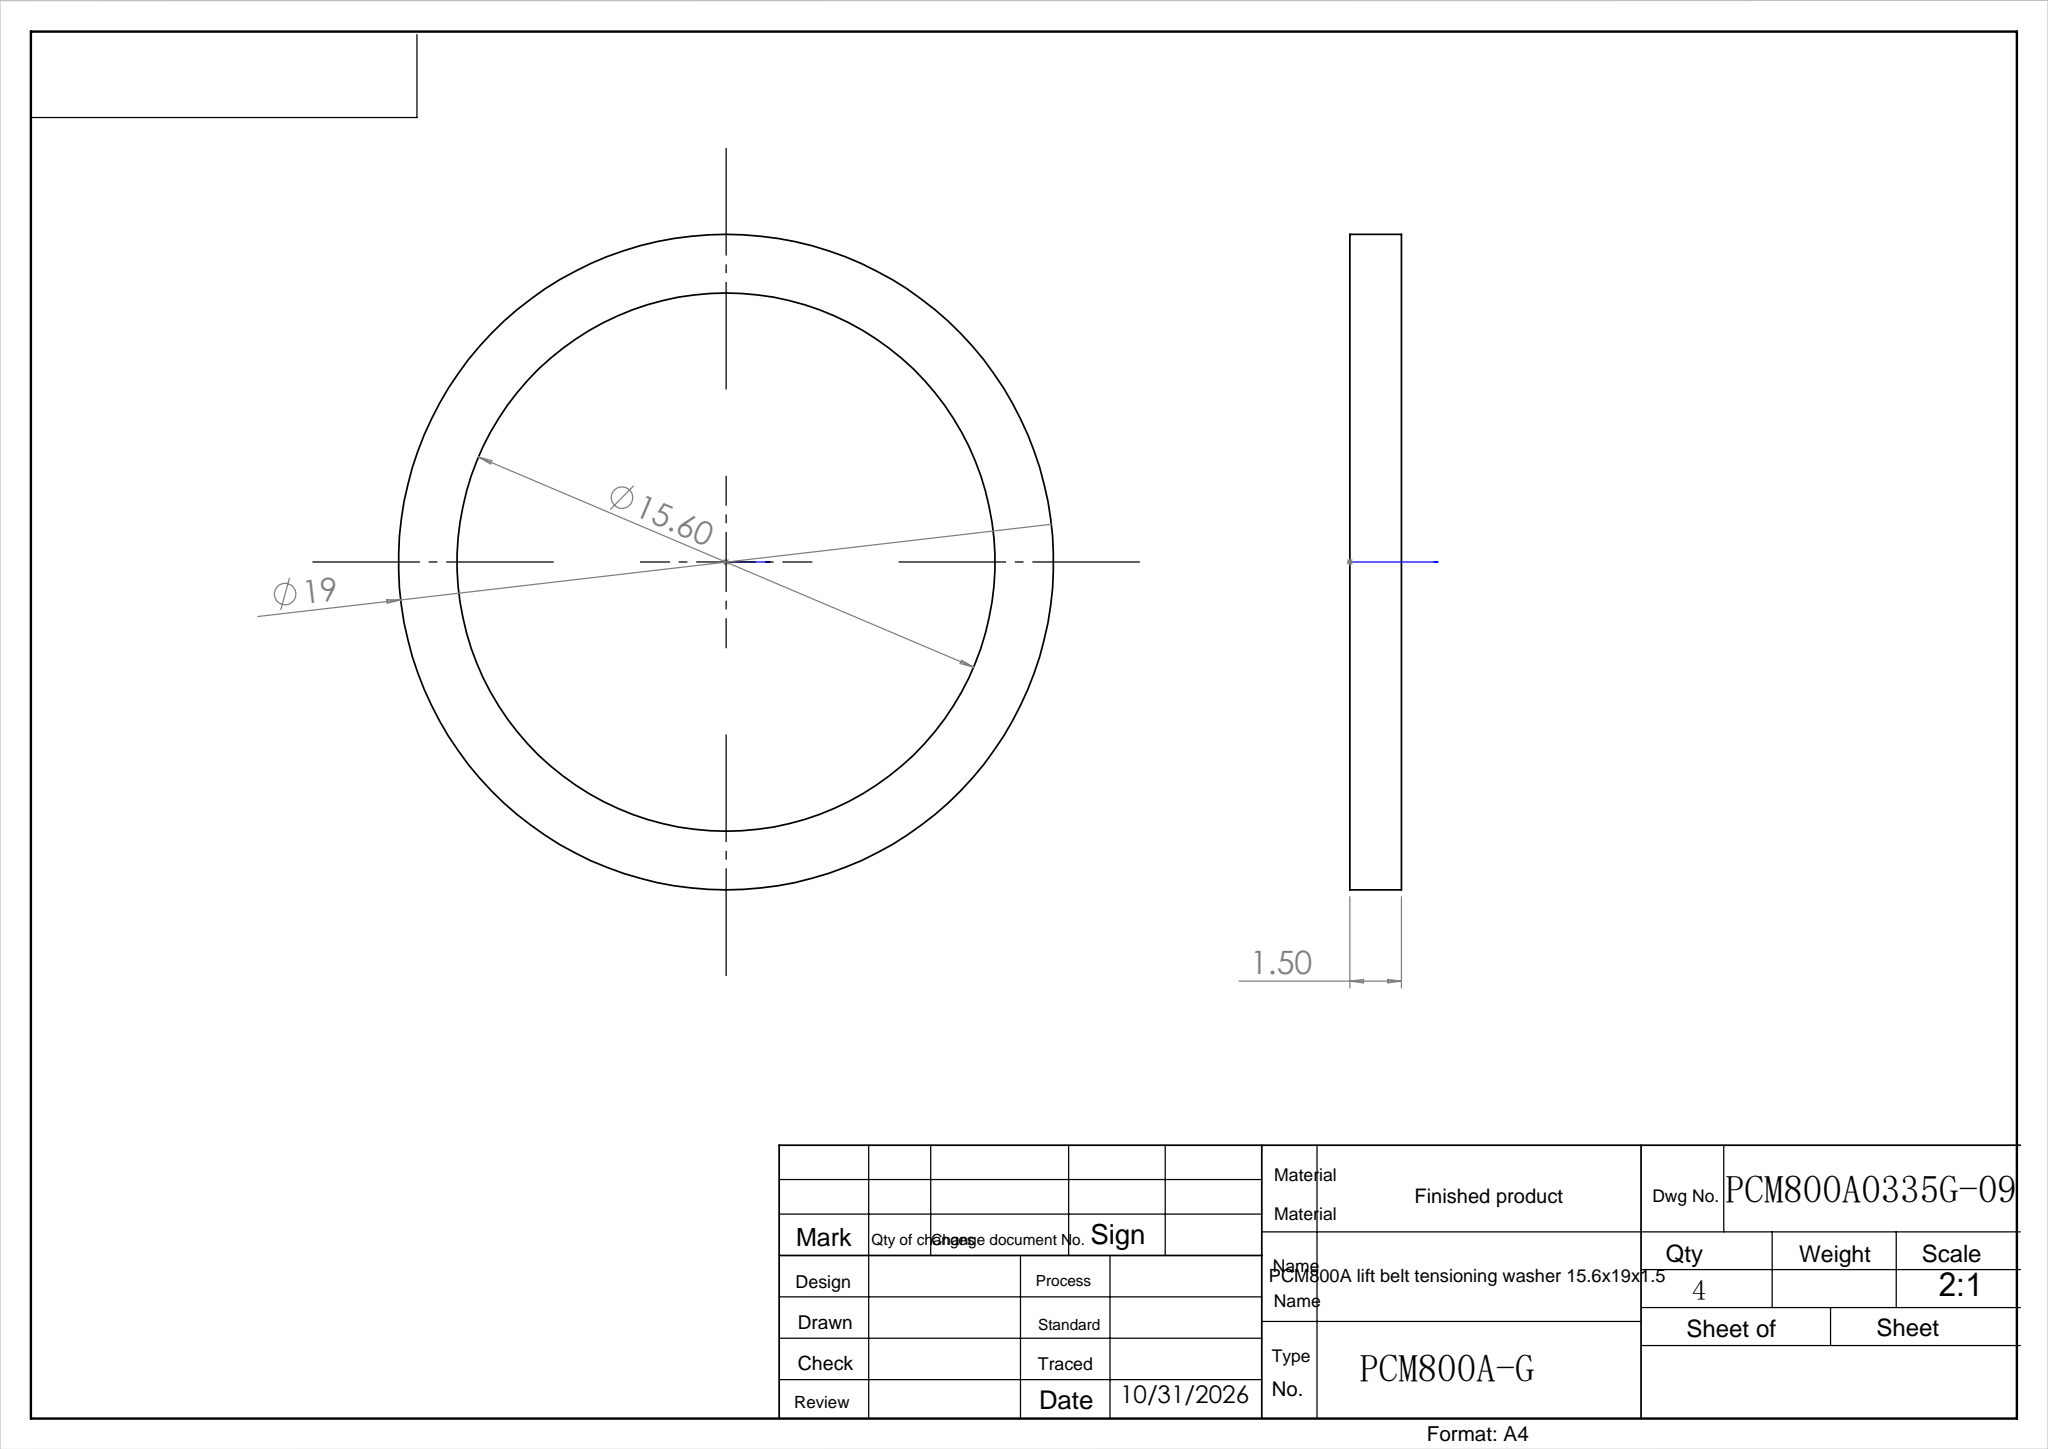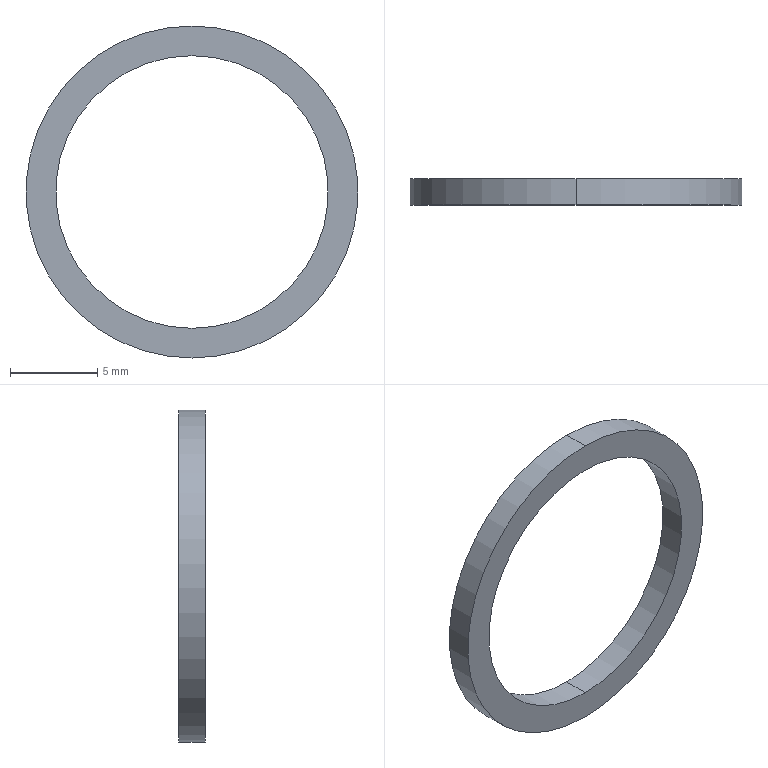Part | SolidWorks | features Extrusion 1 | 1 solid | 6 faces | box 19 x 1.5 x 19 mm | volume 138.591 mm3 | cylinder 4 | plane 2 | commonest cylinder face diameters 15.6 x2 19 x2
STEP:
#1=CARTESIAN_POINT('',(0.,1.5,-7.8));
#2=VERTEX_POINT('',#1);
#3=CARTESIAN_POINT('',(0.,1.5,7.8));
#4=VERTEX_POINT('',#3);
#5=CARTESIAN_POINT('',(0.,1.5,0.));
#6=DIRECTION('',(0.,1.,0.));
#7=DIRECTION('',(0.,0.,1.));
#8=AXIS2_PLACEMENT_3D('',#5,#6,#7);
#9=CIRCLE('',#8,7.8);
#10=EDGE_CURVE('',#2,#4,#9,.T.);
#11=ORIENTED_EDGE('',*,*,#10,.T.);
#12=CARTESIAN_POINT('',(0.,0.,7.8));
#13=VERTEX_POINT('',#12);
#14=CARTESIAN_POINT('',(0.,1.5,7.8));
#15=DIRECTION('',(0.,-1.,0.));
#16=VECTOR('',#15,1000.);
#17=LINE('',#14,#16);
#18=EDGE_CURVE('',#4,#13,#17,.T.);
#19=ORIENTED_EDGE('',*,*,#18,.T.);
#20=CARTESIAN_POINT('',(0.,0.,-7.8));
#21=VERTEX_POINT('',#20);
#22=CARTESIAN_POINT('',(0.,0.,0.));
#23=DIRECTION('',(0.,1.,0.));
#24=DIRECTION('',(0.,0.,1.));
#25=AXIS2_PLACEMENT_3D('',#22,#23,#24);
#26=CIRCLE('',#25,7.8);
#27=EDGE_CURVE('',#21,#13,#26,.T.);
#28=ORIENTED_EDGE('',*,*,#27,.F.);
#29=CARTESIAN_POINT('',(0.,1.5,-7.8));
#30=DIRECTION('',(0.,-1.,0.));
#31=VECTOR('',#30,1000.);
#32=LINE('',#29,#31);
#33=EDGE_CURVE('',#2,#21,#32,.T.);
#34=ORIENTED_EDGE('',*,*,#33,.F.);
#35=EDGE_LOOP('',(#11,#19,#28,#34));
#36=FACE_OUTER_BOUND('',#35,.T.);
#37=CARTESIAN_POINT('',(0.,1.5,0.));
#38=DIRECTION('',(0.,-1.,0.));
#39=DIRECTION('',(0.,0.,-1.));
#40=AXIS2_PLACEMENT_3D('',#37,#38,#39);
#41=CYLINDRICAL_SURFACE('',#40,7.8);
#42=ADVANCED_FACE('',(#36),#41,.F.);
#43=CARTESIAN_POINT('',(0.,1.5,9.5));
#44=VERTEX_POINT('',#43);
#45=CARTESIAN_POINT('',(0.,1.5,-9.5));
#46=VERTEX_POINT('',#45);
#47=CARTESIAN_POINT('',(0.,1.5,0.));
#48=DIRECTION('',(0.,1.,0.));
#49=DIRECTION('',(0.,0.,1.));
#50=AXIS2_PLACEMENT_3D('',#47,#48,#49);
#51=CIRCLE('',#50,9.5);
#52=EDGE_CURVE('',#44,#46,#51,.T.);
#53=ORIENTED_EDGE('',*,*,#52,.F.);
#54=CARTESIAN_POINT('',(0.,0.,9.5));
#55=VERTEX_POINT('',#54);
#56=CARTESIAN_POINT('',(0.,1.5,9.5));
#57=DIRECTION('',(0.,-1.,0.));
#58=VECTOR('',#57,1000.);
#59=LINE('',#56,#58);
#60=EDGE_CURVE('',#44,#55,#59,.T.);
#61=ORIENTED_EDGE('',*,*,#60,.T.);
#62=CARTESIAN_POINT('',(0.,0.,-9.5));
#63=VERTEX_POINT('',#62);
#64=CARTESIAN_POINT('',(0.,0.,0.));
#65=DIRECTION('',(0.,1.,0.));
#66=DIRECTION('',(0.,0.,1.));
#67=AXIS2_PLACEMENT_3D('',#64,#65,#66);
#68=CIRCLE('',#67,9.5);
#69=EDGE_CURVE('',#55,#63,#68,.T.);
#70=ORIENTED_EDGE('',*,*,#69,.T.);
#71=CARTESIAN_POINT('',(0.,1.5,-9.5));
#72=DIRECTION('',(0.,-1.,0.));
#73=VECTOR('',#72,1000.);
#74=LINE('',#71,#73);
#75=EDGE_CURVE('',#46,#63,#74,.T.);
#76=ORIENTED_EDGE('',*,*,#75,.F.);
#77=EDGE_LOOP('',(#53,#61,#70,#76));
#78=FACE_OUTER_BOUND('',#77,.T.);
#79=CARTESIAN_POINT('',(0.,1.5,0.));
#80=DIRECTION('',(0.,-1.,0.));
#81=DIRECTION('',(0.,0.,-1.));
#82=AXIS2_PLACEMENT_3D('',#79,#80,#81);
#83=CYLINDRICAL_SURFACE('',#82,9.5);
#84=ADVANCED_FACE('',(#78),#83,.T.);
#85=CARTESIAN_POINT('',(0.,1.5,0.));
#86=DIRECTION('',(0.,1.,0.));
#87=DIRECTION('',(0.,0.,1.));
#88=AXIS2_PLACEMENT_3D('',#85,#86,#87);
#89=CIRCLE('',#88,9.5);
#90=EDGE_CURVE('',#46,#44,#89,.T.);
#91=ORIENTED_EDGE('',*,*,#90,.T.);
#92=ORIENTED_EDGE('',*,*,#52,.T.);
#93=EDGE_LOOP('',(#91,#92));
#94=FACE_OUTER_BOUND('',#93,.T.);
#95=ORIENTED_EDGE('',*,*,#10,.F.);
#96=CARTESIAN_POINT('',(0.,1.5,0.));
#97=DIRECTION('',(0.,1.,0.));
#98=DIRECTION('',(0.,0.,1.));
#99=AXIS2_PLACEMENT_3D('',#96,#97,#98);
#100=CIRCLE('',#99,7.8);
#101=EDGE_CURVE('',#4,#2,#100,.T.);
#102=ORIENTED_EDGE('',*,*,#101,.F.);
#103=EDGE_LOOP('',(#95,#102));
#104=FACE_BOUND('',#103,.T.);
#105=CARTESIAN_POINT('',(0.,1.5,0.));
#106=DIRECTION('',(0.,1.,0.));
#107=DIRECTION('',(0.,0.,1.));
#108=AXIS2_PLACEMENT_3D('',#105,#106,#107);
#109=PLANE('',#108);
#110=ADVANCED_FACE('',(#94,#104),#109,.T.);
#111=CARTESIAN_POINT('',(0.,0.,0.));
#112=DIRECTION('',(0.,1.,0.));
#113=DIRECTION('',(0.,0.,1.));
#114=AXIS2_PLACEMENT_3D('',#111,#112,#113);
#115=CIRCLE('',#114,9.5);
#116=EDGE_CURVE('',#63,#55,#115,.T.);
#117=ORIENTED_EDGE('',*,*,#116,.F.);
#118=ORIENTED_EDGE('',*,*,#69,.F.);
#119=EDGE_LOOP('',(#117,#118));
#120=FACE_OUTER_BOUND('',#119,.T.);
#121=ORIENTED_EDGE('',*,*,#27,.T.);
#122=CARTESIAN_POINT('',(0.,0.,0.));
#123=DIRECTION('',(0.,1.,0.));
#124=DIRECTION('',(0.,0.,1.));
#125=AXIS2_PLACEMENT_3D('',#122,#123,#124);
#126=CIRCLE('',#125,7.8);
#127=EDGE_CURVE('',#13,#21,#126,.T.);
#128=ORIENTED_EDGE('',*,*,#127,.T.);
#129=EDGE_LOOP('',(#121,#128));
#130=FACE_BOUND('',#129,.T.);
#131=CARTESIAN_POINT('',(0.,0.,0.));
#132=DIRECTION('',(0.,1.,0.));
#133=DIRECTION('',(0.,0.,1.));
#134=AXIS2_PLACEMENT_3D('',#131,#132,#133);
#135=PLANE('',#134);
#136=ADVANCED_FACE('',(#120,#130),#135,.F.);
#137=ORIENTED_EDGE('',*,*,#60,.F.);
#138=ORIENTED_EDGE('',*,*,#90,.F.);
#139=ORIENTED_EDGE('',*,*,#75,.T.);
#140=ORIENTED_EDGE('',*,*,#116,.T.);
#141=EDGE_LOOP('',(#137,#138,#139,#140));
#142=FACE_OUTER_BOUND('',#141,.T.);
#143=CARTESIAN_POINT('',(0.,1.5,0.));
#144=DIRECTION('',(0.,-1.,0.));
#145=DIRECTION('',(0.,0.,-1.));
#146=AXIS2_PLACEMENT_3D('',#143,#144,#145);
#147=CYLINDRICAL_SURFACE('',#146,9.5);
#148=ADVANCED_FACE('',(#142),#147,.T.);
#149=ORIENTED_EDGE('',*,*,#18,.F.);
#150=ORIENTED_EDGE('',*,*,#101,.T.);
#151=ORIENTED_EDGE('',*,*,#33,.T.);
#152=ORIENTED_EDGE('',*,*,#127,.F.);
#153=EDGE_LOOP('',(#149,#150,#151,#152));
#154=FACE_OUTER_BOUND('',#153,.T.);
#155=CARTESIAN_POINT('',(0.,1.5,0.));
#156=DIRECTION('',(0.,-1.,0.));
#157=DIRECTION('',(0.,0.,-1.));
#158=AXIS2_PLACEMENT_3D('',#155,#156,#157);
#159=CYLINDRICAL_SURFACE('',#158,7.8);
#160=ADVANCED_FACE('',(#154),#159,.F.);
#161=CLOSED_SHELL('',(#42,#84,#110,#136,#148,#160));
#162=MANIFOLD_SOLID_BREP('',#161);
#163=CARTESIAN_POINT('',(0.,0.,0.));
#164=DIRECTION('',(0.,0.,1.));
#165=DIRECTION('',(1.,0.,0.));
#166=AXIS2_PLACEMENT_3D('',#163,#164,#165);
#167=(LENGTH_UNIT()NAMED_UNIT(*)SI_UNIT(.MILLI.,.METRE.));
#168=UNCERTAINTY_MEASURE_WITH_UNIT(LENGTH_MEASURE(0.00001),#167,'','');
#169=(NAMED_UNIT(*)PLANE_ANGLE_UNIT()SI_UNIT($,.RADIAN.));
#170=(NAMED_UNIT(*)SI_UNIT($,.STERADIAN.)SOLID_ANGLE_UNIT());
#171=(GEOMETRIC_REPRESENTATION_CONTEXT(3)GLOBAL_UNCERTAINTY_ASSIGNED_CONTEXT((#168))GLOBAL_UNIT_ASSIGNED_CONTEXT((#167,#169,#170))REPRESENTATION_CONTEXT('',''));
#172=ADVANCED_BREP_SHAPE_REPRESENTATION('',(#162,#166),#171);